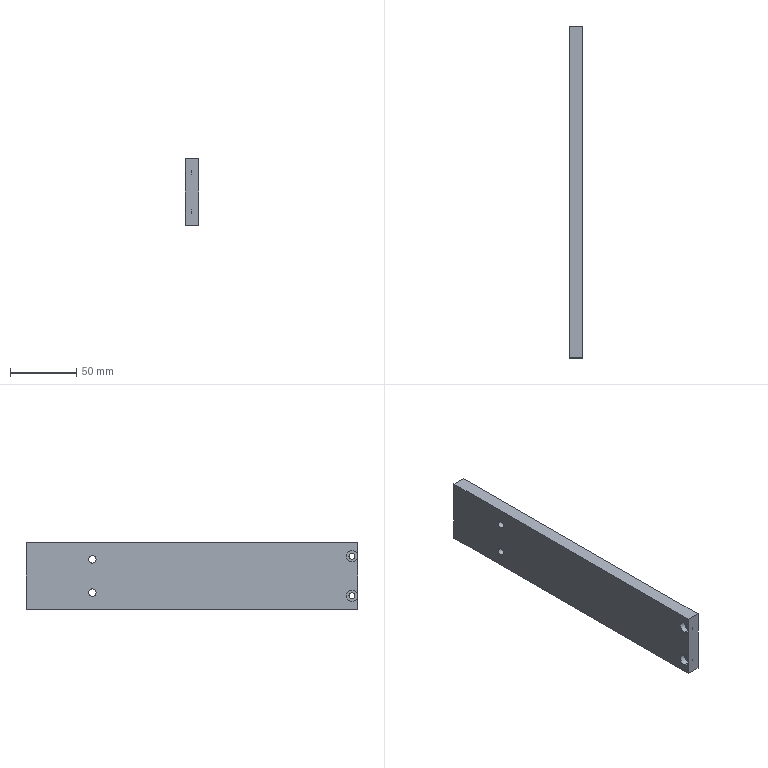Part | STEP file | 01-12 Coil feed support plate | 1 solid | 20 faces | box 10 x 250 x 50 mm | volume 123839 mm3 | cylinder 12 | plane 8 | commonest cylinder face diameters 4.5 x4 5.5 x4 8.5 x4